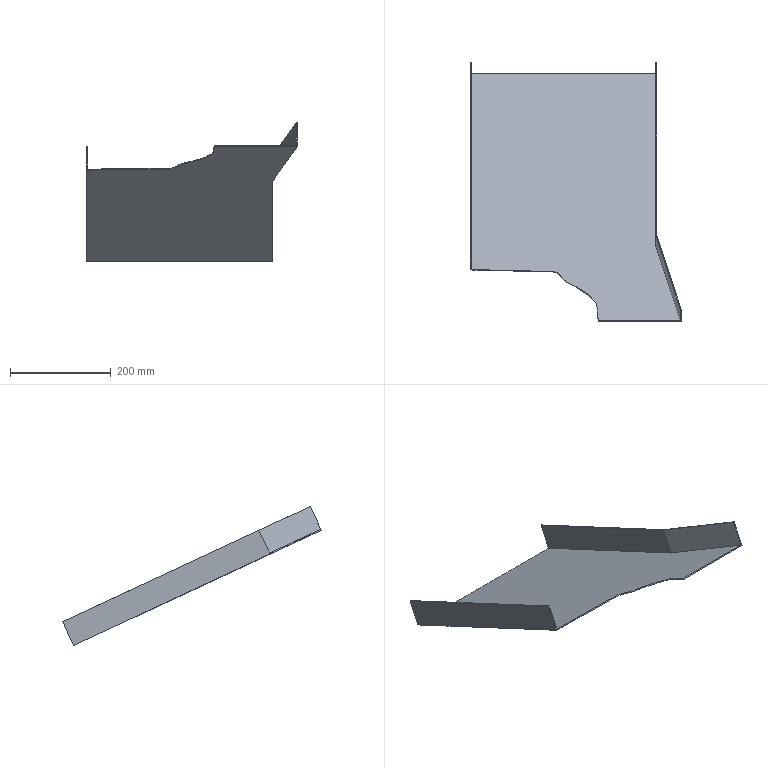Part | NX | features solid 2 | 1 solid | 13 faces | box 418.838 x 513.626 x 276.388 mm | volume 476232 mm3 | plane 12 | spline 1